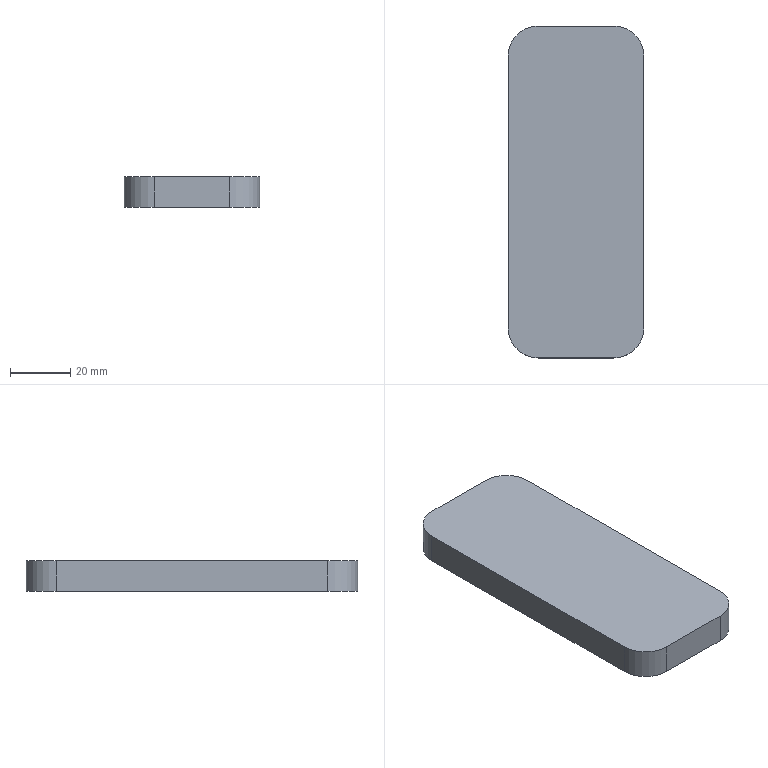Part | STEP file | SL2-MOLD_id14_xmt_txt | 1 solid | 10 faces | box 45 x 110 x 10 mm | volume 48642 mm3 | plane 6 | cylinder 4 | commonest cylinder face diameters 20 x4
STEP:
#1=CARTESIAN_POINT('',(-190.,45.,20.));
#2=VERTEX_POINT('',#1);
#3=CARTESIAN_POINT('',(-190.,135.,20.));
#4=VERTEX_POINT('',#3);
#5=CARTESIAN_POINT('',(-190.,35.,20.));
#6=DIRECTION('',(0.,1.,0.));
#7=VECTOR('',#6,1.);
#8=LINE('',#5,#7);
#9=EDGE_CURVE('',#2,#4,#8,.T.);
#10=ORIENTED_EDGE('',*,*,#9,.F.);
#11=CARTESIAN_POINT('',(-190.,45.,30.));
#12=VERTEX_POINT('',#11);
#13=CARTESIAN_POINT('',(-190.,45.,20.));
#14=DIRECTION('',(0.,0.,1.));
#15=VECTOR('',#14,1.);
#16=LINE('',#13,#15);
#17=EDGE_CURVE('',#2,#12,#16,.T.);
#18=ORIENTED_EDGE('',*,*,#17,.T.);
#19=CARTESIAN_POINT('',(-190.,135.,30.));
#20=VERTEX_POINT('',#19);
#21=CARTESIAN_POINT('',(-190.,35.,30.));
#22=DIRECTION('',(0.,1.,0.));
#23=VECTOR('',#22,1.);
#24=LINE('',#21,#23);
#25=EDGE_CURVE('',#12,#20,#24,.T.);
#26=ORIENTED_EDGE('',*,*,#25,.T.);
#27=CARTESIAN_POINT('',(-190.,135.,20.));
#28=DIRECTION('',(0.,0.,-1.));
#29=VECTOR('',#28,1.);
#30=LINE('',#27,#29);
#31=EDGE_CURVE('',#20,#4,#30,.T.);
#32=ORIENTED_EDGE('',*,*,#31,.T.);
#33=EDGE_LOOP('',(#10,#18,#26,#32));
#34=FACE_OUTER_BOUND('',#33,.T.);
#35=CARTESIAN_POINT('',(-190.,35.,20.));
#36=DIRECTION('',(1.,0.,0.));
#37=DIRECTION('',(0.,0.,-1.));
#38=AXIS2_PLACEMENT_3D('',#35,#36,#37);
#39=PLANE('',#38);
#40=ADVANCED_FACE('',(#34),#39,.F.);
#41=CARTESIAN_POINT('',(-180.,145.,30.));
#42=VERTEX_POINT('',#41);
#43=CARTESIAN_POINT('',(-155.,145.,30.));
#44=VERTEX_POINT('',#43);
#45=CARTESIAN_POINT('',(-190.,145.,30.));
#46=DIRECTION('',(1.,0.,0.));
#47=VECTOR('',#46,1.);
#48=LINE('',#45,#47);
#49=EDGE_CURVE('',#42,#44,#48,.T.);
#50=ORIENTED_EDGE('',*,*,#49,.T.);
#51=CARTESIAN_POINT('',(-155.,145.,20.));
#52=VERTEX_POINT('',#51);
#53=CARTESIAN_POINT('',(-155.,145.,20.));
#54=DIRECTION('',(0.,0.,-1.));
#55=VECTOR('',#54,1.);
#56=LINE('',#53,#55);
#57=EDGE_CURVE('',#44,#52,#56,.T.);
#58=ORIENTED_EDGE('',*,*,#57,.T.);
#59=CARTESIAN_POINT('',(-180.,145.,20.));
#60=VERTEX_POINT('',#59);
#61=CARTESIAN_POINT('',(-190.,145.,20.));
#62=DIRECTION('',(1.,0.,0.));
#63=VECTOR('',#62,1.);
#64=LINE('',#61,#63);
#65=EDGE_CURVE('',#60,#52,#64,.T.);
#66=ORIENTED_EDGE('',*,*,#65,.F.);
#67=CARTESIAN_POINT('',(-180.,145.,20.));
#68=DIRECTION('',(0.,0.,1.));
#69=VECTOR('',#68,1.);
#70=LINE('',#67,#69);
#71=EDGE_CURVE('',#60,#42,#70,.T.);
#72=ORIENTED_EDGE('',*,*,#71,.T.);
#73=EDGE_LOOP('',(#50,#58,#66,#72));
#74=FACE_OUTER_BOUND('',#73,.T.);
#75=CARTESIAN_POINT('',(-190.,145.,20.));
#76=DIRECTION('',(0.,-1.,0.));
#77=DIRECTION('',(0.,0.,-1.));
#78=AXIS2_PLACEMENT_3D('',#75,#76,#77);
#79=PLANE('',#78);
#80=ADVANCED_FACE('',(#74),#79,.F.);
#81=CARTESIAN_POINT('',(-145.,135.,30.));
#82=VERTEX_POINT('',#81);
#83=CARTESIAN_POINT('',(-145.,45.,30.));
#84=VERTEX_POINT('',#83);
#85=CARTESIAN_POINT('',(-145.,145.,30.));
#86=DIRECTION('',(0.,-1.,0.));
#87=VECTOR('',#86,1.);
#88=LINE('',#85,#87);
#89=EDGE_CURVE('',#82,#84,#88,.T.);
#90=ORIENTED_EDGE('',*,*,#89,.T.);
#91=CARTESIAN_POINT('',(-145.,45.,20.));
#92=VERTEX_POINT('',#91);
#93=CARTESIAN_POINT('',(-145.,45.,20.));
#94=DIRECTION('',(0.,0.,-1.));
#95=VECTOR('',#94,1.);
#96=LINE('',#93,#95);
#97=EDGE_CURVE('',#84,#92,#96,.T.);
#98=ORIENTED_EDGE('',*,*,#97,.T.);
#99=CARTESIAN_POINT('',(-145.,135.,20.));
#100=VERTEX_POINT('',#99);
#101=CARTESIAN_POINT('',(-145.,145.,20.));
#102=DIRECTION('',(0.,-1.,0.));
#103=VECTOR('',#102,1.);
#104=LINE('',#101,#103);
#105=EDGE_CURVE('',#100,#92,#104,.T.);
#106=ORIENTED_EDGE('',*,*,#105,.F.);
#107=CARTESIAN_POINT('',(-145.,135.,20.));
#108=DIRECTION('',(0.,0.,1.));
#109=VECTOR('',#108,1.);
#110=LINE('',#107,#109);
#111=EDGE_CURVE('',#100,#82,#110,.T.);
#112=ORIENTED_EDGE('',*,*,#111,.T.);
#113=EDGE_LOOP('',(#90,#98,#106,#112));
#114=FACE_OUTER_BOUND('',#113,.T.);
#115=CARTESIAN_POINT('',(-145.,145.,20.));
#116=DIRECTION('',(-1.,0.,0.));
#117=DIRECTION('',(0.,0.,1.));
#118=AXIS2_PLACEMENT_3D('',#115,#116,#117);
#119=PLANE('',#118);
#120=ADVANCED_FACE('',(#114),#119,.F.);
#121=CARTESIAN_POINT('',(-155.,35.,20.));
#122=VERTEX_POINT('',#121);
#123=CARTESIAN_POINT('',(-180.,35.,20.));
#124=VERTEX_POINT('',#123);
#125=CARTESIAN_POINT('',(-145.,35.,20.));
#126=DIRECTION('',(-1.,0.,0.));
#127=VECTOR('',#126,1.);
#128=LINE('',#125,#127);
#129=EDGE_CURVE('',#122,#124,#128,.T.);
#130=ORIENTED_EDGE('',*,*,#129,.F.);
#131=CARTESIAN_POINT('',(-155.,35.,30.));
#132=VERTEX_POINT('',#131);
#133=CARTESIAN_POINT('',(-155.,35.,20.));
#134=DIRECTION('',(0.,0.,1.));
#135=VECTOR('',#134,1.);
#136=LINE('',#133,#135);
#137=EDGE_CURVE('',#122,#132,#136,.T.);
#138=ORIENTED_EDGE('',*,*,#137,.T.);
#139=CARTESIAN_POINT('',(-180.,35.,30.));
#140=VERTEX_POINT('',#139);
#141=CARTESIAN_POINT('',(-145.,35.,30.));
#142=DIRECTION('',(-1.,0.,0.));
#143=VECTOR('',#142,1.);
#144=LINE('',#141,#143);
#145=EDGE_CURVE('',#132,#140,#144,.T.);
#146=ORIENTED_EDGE('',*,*,#145,.T.);
#147=CARTESIAN_POINT('',(-180.,35.,20.));
#148=DIRECTION('',(0.,0.,-1.));
#149=VECTOR('',#148,1.);
#150=LINE('',#147,#149);
#151=EDGE_CURVE('',#140,#124,#150,.T.);
#152=ORIENTED_EDGE('',*,*,#151,.T.);
#153=EDGE_LOOP('',(#130,#138,#146,#152));
#154=FACE_OUTER_BOUND('',#153,.T.);
#155=CARTESIAN_POINT('',(-145.,35.,20.));
#156=DIRECTION('',(0.,1.,0.));
#157=DIRECTION('',(0.,0.,1.));
#158=AXIS2_PLACEMENT_3D('',#155,#156,#157);
#159=PLANE('',#158);
#160=ADVANCED_FACE('',(#154),#159,.F.);
#161=ORIENTED_EDGE('',*,*,#105,.T.);
#162=CARTESIAN_POINT('',(-155.,45.,20.));
#163=DIRECTION('',(0.,0.,-1.));
#164=DIRECTION('',(-1.,0.,0.));
#165=AXIS2_PLACEMENT_3D('',#162,#163,#164);
#166=CIRCLE('',#165,10.);
#167=EDGE_CURVE('',#92,#122,#166,.T.);
#168=ORIENTED_EDGE('',*,*,#167,.T.);
#169=ORIENTED_EDGE('',*,*,#129,.T.);
#170=CARTESIAN_POINT('',(-180.,45.,20.));
#171=DIRECTION('',(0.,0.,-1.));
#172=DIRECTION('',(-1.,0.,0.));
#173=AXIS2_PLACEMENT_3D('',#170,#171,#172);
#174=CIRCLE('',#173,10.);
#175=EDGE_CURVE('',#124,#2,#174,.T.);
#176=ORIENTED_EDGE('',*,*,#175,.T.);
#177=ORIENTED_EDGE('',*,*,#9,.T.);
#178=CARTESIAN_POINT('',(-180.,135.,20.));
#179=DIRECTION('',(0.,0.,-1.));
#180=DIRECTION('',(-1.,0.,0.));
#181=AXIS2_PLACEMENT_3D('',#178,#179,#180);
#182=CIRCLE('',#181,10.);
#183=EDGE_CURVE('',#4,#60,#182,.T.);
#184=ORIENTED_EDGE('',*,*,#183,.T.);
#185=ORIENTED_EDGE('',*,*,#65,.T.);
#186=CARTESIAN_POINT('',(-155.,135.,20.));
#187=DIRECTION('',(0.,0.,-1.));
#188=DIRECTION('',(-1.,0.,0.));
#189=AXIS2_PLACEMENT_3D('',#186,#187,#188);
#190=CIRCLE('',#189,10.);
#191=EDGE_CURVE('',#52,#100,#190,.T.);
#192=ORIENTED_EDGE('',*,*,#191,.T.);
#193=EDGE_LOOP('',(#161,#168,#169,#176,#177,#184,#185,#192));
#194=FACE_OUTER_BOUND('',#193,.T.);
#195=CARTESIAN_POINT('',(0.,0.,20.));
#196=DIRECTION('',(0.,0.,-1.));
#197=DIRECTION('',(-1.,0.,0.));
#198=AXIS2_PLACEMENT_3D('',#195,#196,#197);
#199=PLANE('',#198);
#200=ADVANCED_FACE('',(#194),#199,.T.);
#201=ORIENTED_EDGE('',*,*,#145,.F.);
#202=CARTESIAN_POINT('',(-155.,45.,30.));
#203=DIRECTION('',(0.,0.,1.));
#204=DIRECTION('',(-1.,0.,0.));
#205=AXIS2_PLACEMENT_3D('',#202,#203,#204);
#206=CIRCLE('',#205,10.);
#207=EDGE_CURVE('',#132,#84,#206,.T.);
#208=ORIENTED_EDGE('',*,*,#207,.T.);
#209=ORIENTED_EDGE('',*,*,#89,.F.);
#210=CARTESIAN_POINT('',(-155.,135.,30.));
#211=DIRECTION('',(0.,0.,1.));
#212=DIRECTION('',(-1.,0.,0.));
#213=AXIS2_PLACEMENT_3D('',#210,#211,#212);
#214=CIRCLE('',#213,10.);
#215=EDGE_CURVE('',#82,#44,#214,.T.);
#216=ORIENTED_EDGE('',*,*,#215,.T.);
#217=ORIENTED_EDGE('',*,*,#49,.F.);
#218=CARTESIAN_POINT('',(-180.,135.,30.));
#219=DIRECTION('',(0.,0.,1.));
#220=DIRECTION('',(-1.,0.,0.));
#221=AXIS2_PLACEMENT_3D('',#218,#219,#220);
#222=CIRCLE('',#221,10.);
#223=EDGE_CURVE('',#42,#20,#222,.T.);
#224=ORIENTED_EDGE('',*,*,#223,.T.);
#225=ORIENTED_EDGE('',*,*,#25,.F.);
#226=CARTESIAN_POINT('',(-180.,45.,30.));
#227=DIRECTION('',(0.,0.,1.));
#228=DIRECTION('',(-1.,0.,0.));
#229=AXIS2_PLACEMENT_3D('',#226,#227,#228);
#230=CIRCLE('',#229,10.);
#231=EDGE_CURVE('',#12,#140,#230,.T.);
#232=ORIENTED_EDGE('',*,*,#231,.T.);
#233=EDGE_LOOP('',(#201,#208,#209,#216,#217,#224,#225,#232));
#234=FACE_OUTER_BOUND('',#233,.T.);
#235=CARTESIAN_POINT('',(0.,0.,30.));
#236=DIRECTION('',(0.,0.,-1.));
#237=DIRECTION('',(-1.,0.,0.));
#238=AXIS2_PLACEMENT_3D('',#235,#236,#237);
#239=PLANE('',#238);
#240=ADVANCED_FACE('',(#234),#239,.F.);
#241=ORIENTED_EDGE('',*,*,#167,.F.);
#242=ORIENTED_EDGE('',*,*,#97,.F.);
#243=ORIENTED_EDGE('',*,*,#207,.F.);
#244=ORIENTED_EDGE('',*,*,#137,.F.);
#245=EDGE_LOOP('',(#241,#242,#243,#244));
#246=FACE_OUTER_BOUND('',#245,.T.);
#247=CARTESIAN_POINT('',(-155.,45.,20.));
#248=DIRECTION('',(0.,0.,1.));
#249=DIRECTION('',(1.,0.,0.));
#250=AXIS2_PLACEMENT_3D('',#247,#248,#249);
#251=CYLINDRICAL_SURFACE('',#250,10.);
#252=ADVANCED_FACE('',(#246),#251,.T.);
#253=ORIENTED_EDGE('',*,*,#175,.F.);
#254=ORIENTED_EDGE('',*,*,#151,.F.);
#255=ORIENTED_EDGE('',*,*,#231,.F.);
#256=ORIENTED_EDGE('',*,*,#17,.F.);
#257=EDGE_LOOP('',(#253,#254,#255,#256));
#258=FACE_OUTER_BOUND('',#257,.T.);
#259=CARTESIAN_POINT('',(-180.,45.,20.));
#260=DIRECTION('',(0.,0.,1.));
#261=DIRECTION('',(1.,0.,0.));
#262=AXIS2_PLACEMENT_3D('',#259,#260,#261);
#263=CYLINDRICAL_SURFACE('',#262,10.);
#264=ADVANCED_FACE('',(#258),#263,.T.);
#265=ORIENTED_EDGE('',*,*,#191,.F.);
#266=ORIENTED_EDGE('',*,*,#57,.F.);
#267=ORIENTED_EDGE('',*,*,#215,.F.);
#268=ORIENTED_EDGE('',*,*,#111,.F.);
#269=EDGE_LOOP('',(#265,#266,#267,#268));
#270=FACE_OUTER_BOUND('',#269,.T.);
#271=CARTESIAN_POINT('',(-155.,135.,20.));
#272=DIRECTION('',(0.,0.,1.));
#273=DIRECTION('',(1.,0.,0.));
#274=AXIS2_PLACEMENT_3D('',#271,#272,#273);
#275=CYLINDRICAL_SURFACE('',#274,10.);
#276=ADVANCED_FACE('',(#270),#275,.T.);
#277=ORIENTED_EDGE('',*,*,#183,.F.);
#278=ORIENTED_EDGE('',*,*,#31,.F.);
#279=ORIENTED_EDGE('',*,*,#223,.F.);
#280=ORIENTED_EDGE('',*,*,#71,.F.);
#281=EDGE_LOOP('',(#277,#278,#279,#280));
#282=FACE_OUTER_BOUND('',#281,.T.);
#283=CARTESIAN_POINT('',(-180.,135.,20.));
#284=DIRECTION('',(0.,0.,1.));
#285=DIRECTION('',(1.,0.,0.));
#286=AXIS2_PLACEMENT_3D('',#283,#284,#285);
#287=CYLINDRICAL_SURFACE('',#286,10.);
#288=ADVANCED_FACE('',(#282),#287,.T.);
#289=CLOSED_SHELL('',(#40,#80,#120,#160,#200,#240,#252,#264,#276,#288));
#290=MANIFOLD_SOLID_BREP('',#289);
#291=(LENGTH_UNIT()NAMED_UNIT(*)SI_UNIT(.MILLI.,.METRE.));
#292=UNCERTAINTY_MEASURE_WITH_UNIT(LENGTH_MEASURE(0.00002),#291,'','');
#293=(NAMED_UNIT(*)PLANE_ANGLE_UNIT()SI_UNIT($,.RADIAN.));
#294=PLANE_ANGLE_MEASURE_WITH_UNIT(PLANE_ANGLE_MEASURE(0.01745),#293);
#295=DIMENSIONAL_EXPONENTS(0.,0.,0.,0.,0.,0.,0.);
#296=(CONVERSION_BASED_UNIT('DEGREE',#294)NAMED_UNIT(#295)PLANE_ANGLE_UNIT());
#297=(NAMED_UNIT(*)SI_UNIT($,.STERADIAN.)SOLID_ANGLE_UNIT());
#298=(GEOMETRIC_REPRESENTATION_CONTEXT(3)GLOBAL_UNCERTAINTY_ASSIGNED_CONTEXT((#292))GLOBAL_UNIT_ASSIGNED_CONTEXT((#291,#296,#297))REPRESENTATION_CONTEXT('',''));
#299=ADVANCED_BREP_SHAPE_REPRESENTATION('',(#290),#298);